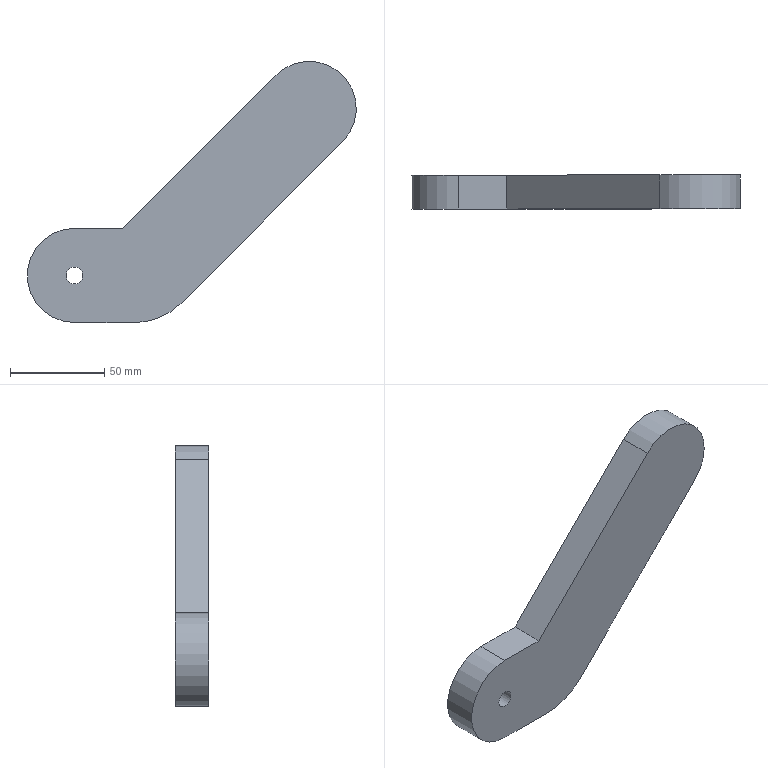Part | STEP file | Leg_right | 1 solid | 10 faces | box 174.595 x 18 x 138.64 mm | volume 178903 mm3 | plane 6 | cylinder 4 | commonest cylinder face diameters 50 x2 9 x1 70 x1
STEP:
#1=CARTESIAN_POINT('',(0.,0.,0.));
#2=DIRECTION('',(0.,0.,1.));
#3=DIRECTION('',(1.,0.,0.));
#4=AXIS2_PLACEMENT_3D('',#1,#2,#3);
#5=CARTESIAN_POINT('',(0.,0.,25.));
#6=VERTEX_POINT('',#5);
#7=CARTESIAN_POINT('',(0.,0.,-25.));
#8=VERTEX_POINT('',#7);
#9=CARTESIAN_POINT('',(0.,0.,0.));
#10=DIRECTION('',(0.,-1.,0.));
#11=DIRECTION('',(1.,0.,0.));
#12=AXIS2_PLACEMENT_3D('',#9,#10,#11);
#13=CIRCLE('',#12,25.);
#14=CARTESIAN_POINT('',(0.,0.,0.));
#15=DIRECTION('',(0.,1.,0.));
#16=DIRECTION('',(1.,0.,0.));
#17=AXIS2_PLACEMENT_3D('',#14,#15,#16);
#18=CYLINDRICAL_SURFACE('',#17,25.);
#19=CARTESIAN_POINT('',(6.283,0.));
#20=DIRECTION('',(-1.,0.));
#21=VECTOR('',#20,1.);
#22=LINE('',#19,#21);
#23=(GEOMETRIC_REPRESENTATION_CONTEXT(2)PARAMETRIC_REPRESENTATION_CONTEXT()REPRESENTATION_CONTEXT('',''));
#24=DEFINITIONAL_REPRESENTATION('',(#22),#23);
#25=PCURVE('',#18,#24);
#26=CARTESIAN_POINT('',(62.213,0.,35.66));
#27=DIRECTION('',(0.,1.,0.));
#28=DIRECTION('',(0.,0.,1.));
#29=AXIS2_PLACEMENT_3D('',#26,#27,#28);
#30=PLANE('',#29);
#31=CARTESIAN_POINT('',(-35.66,-37.213));
#32=CARTESIAN_POINT('',(7.641,-37.213));
#33=CARTESIAN_POINT('',(-14.009,-74.713));
#34=CARTESIAN_POINT('',(-35.66,-112.213));
#35=CARTESIAN_POINT('',(-57.311,-74.713));
#36=CARTESIAN_POINT('',(-78.961,-37.213));
#37=CARTESIAN_POINT('',(-35.66,-37.213));
#38=(BOUNDED_CURVE()B_SPLINE_CURVE(2,(#31,#32,#33,#34,#35,#36,#37),.UNSPECIFIED.,.T.,.F.)B_SPLINE_CURVE_WITH_KNOTS((1,2,2,2,2,1),(-2.094,0.,2.094,4.189,6.283,8.378),.UNSPECIFIED.)CURVE()GEOMETRIC_REPRESENTATION_ITEM()RATIONAL_B_SPLINE_CURVE((1.,0.5,1.,0.5,1.,0.5,1.))REPRESENTATION_ITEM(''));
#39=(GEOMETRIC_REPRESENTATION_CONTEXT(2)PARAMETRIC_REPRESENTATION_CONTEXT()REPRESENTATION_CONTEXT('',''));
#40=DEFINITIONAL_REPRESENTATION('',(#38),#39);
#41=PCURVE('',#30,#40);
#42=SURFACE_CURVE('',#13,(#25,#41),.PCURVE_S1.);
#43=EDGE_CURVE('',#6,#8,#42,.T.);
#44=ORIENTED_EDGE('',*,*,#43,.T.);
#45=CARTESIAN_POINT('',(0.,-18.,-25.));
#46=VERTEX_POINT('',#45);
#47=CARTESIAN_POINT('',(0.,0.,-25.));
#48=DIRECTION('',(0.,-1.,0.));
#49=VECTOR('',#48,1.);
#50=LINE('',#47,#49);
#51=CARTESIAN_POINT('',(1.571,0.));
#52=DIRECTION('',(0.,-1.));
#53=VECTOR('',#52,1.);
#54=LINE('',#51,#53);
#55=(GEOMETRIC_REPRESENTATION_CONTEXT(2)PARAMETRIC_REPRESENTATION_CONTEXT()REPRESENTATION_CONTEXT('',''));
#56=DEFINITIONAL_REPRESENTATION('',(#54),#55);
#57=PCURVE('',#18,#56);
#58=CARTESIAN_POINT('',(31.813,0.,-25.));
#59=DIRECTION('',(0.,0.,-1.));
#60=DIRECTION('',(-1.,0.,0.));
#61=AXIS2_PLACEMENT_3D('',#58,#59,#60);
#62=PLANE('',#61);
#63=CARTESIAN_POINT('',(31.813,0.));
#64=DIRECTION('',(0.,-1.));
#65=VECTOR('',#64,1.);
#66=LINE('',#63,#65);
#67=(GEOMETRIC_REPRESENTATION_CONTEXT(2)PARAMETRIC_REPRESENTATION_CONTEXT()REPRESENTATION_CONTEXT('',''));
#68=DEFINITIONAL_REPRESENTATION('',(#66),#67);
#69=PCURVE('',#62,#68);
#70=SURFACE_CURVE('',#50,(#57,#69),.PCURVE_S1.);
#71=EDGE_CURVE('',#8,#46,#70,.T.);
#72=ORIENTED_EDGE('',*,*,#71,.T.);
#73=CARTESIAN_POINT('',(0.,-18.,25.));
#74=VERTEX_POINT('',#73);
#75=CARTESIAN_POINT('',(0.,-18.,0.));
#76=DIRECTION('',(0.,-1.,0.));
#77=DIRECTION('',(1.,0.,0.));
#78=AXIS2_PLACEMENT_3D('',#75,#76,#77);
#79=CIRCLE('',#78,25.);
#80=CARTESIAN_POINT('',(6.283,-18.));
#81=DIRECTION('',(-1.,0.));
#82=VECTOR('',#81,1.);
#83=LINE('',#80,#82);
#84=(GEOMETRIC_REPRESENTATION_CONTEXT(2)PARAMETRIC_REPRESENTATION_CONTEXT()REPRESENTATION_CONTEXT('',''));
#85=DEFINITIONAL_REPRESENTATION('',(#83),#84);
#86=PCURVE('',#18,#85);
#87=CARTESIAN_POINT('',(62.213,-18.,35.66));
#88=DIRECTION('',(0.,1.,0.));
#89=DIRECTION('',(0.,0.,1.));
#90=AXIS2_PLACEMENT_3D('',#87,#88,#89);
#91=PLANE('',#90);
#92=CARTESIAN_POINT('',(-35.66,-37.213));
#93=CARTESIAN_POINT('',(7.641,-37.213));
#94=CARTESIAN_POINT('',(-14.009,-74.713));
#95=CARTESIAN_POINT('',(-35.66,-112.213));
#96=CARTESIAN_POINT('',(-57.311,-74.713));
#97=CARTESIAN_POINT('',(-78.961,-37.213));
#98=CARTESIAN_POINT('',(-35.66,-37.213));
#99=(BOUNDED_CURVE()B_SPLINE_CURVE(2,(#92,#93,#94,#95,#96,#97,#98),.UNSPECIFIED.,.T.,.F.)B_SPLINE_CURVE_WITH_KNOTS((1,2,2,2,2,1),(-2.094,0.,2.094,4.189,6.283,8.378),.UNSPECIFIED.)CURVE()GEOMETRIC_REPRESENTATION_ITEM()RATIONAL_B_SPLINE_CURVE((1.,0.5,1.,0.5,1.,0.5,1.))REPRESENTATION_ITEM(''));
#100=(GEOMETRIC_REPRESENTATION_CONTEXT(2)PARAMETRIC_REPRESENTATION_CONTEXT()REPRESENTATION_CONTEXT('',''));
#101=DEFINITIONAL_REPRESENTATION('',(#99),#100);
#102=PCURVE('',#91,#101);
#103=SURFACE_CURVE('',#79,(#86,#102),.PCURVE_S1.);
#104=EDGE_CURVE('',#74,#46,#103,.T.);
#105=ORIENTED_EDGE('',*,*,#104,.F.);
#106=CARTESIAN_POINT('',(0.,0.,25.));
#107=DIRECTION('',(0.,-1.,0.));
#108=VECTOR('',#107,1.);
#109=LINE('',#106,#108);
#110=CARTESIAN_POINT('',(4.712,0.));
#111=DIRECTION('',(0.,-1.));
#112=VECTOR('',#111,1.);
#113=LINE('',#110,#112);
#114=(GEOMETRIC_REPRESENTATION_CONTEXT(2)PARAMETRIC_REPRESENTATION_CONTEXT()REPRESENTATION_CONTEXT('',''));
#115=DEFINITIONAL_REPRESENTATION('',(#113),#114);
#116=PCURVE('',#18,#115);
#117=CARTESIAN_POINT('',(0.,0.,25.));
#118=DIRECTION('',(0.,0.,1.));
#119=DIRECTION('',(1.,0.,0.));
#120=AXIS2_PLACEMENT_3D('',#117,#118,#119);
#121=PLANE('',#120);
#122=CARTESIAN_POINT('',(0.,0.));
#123=DIRECTION('',(0.,-1.));
#124=VECTOR('',#123,1.);
#125=LINE('',#122,#124);
#126=(GEOMETRIC_REPRESENTATION_CONTEXT(2)PARAMETRIC_REPRESENTATION_CONTEXT()REPRESENTATION_CONTEXT('',''));
#127=DEFINITIONAL_REPRESENTATION('',(#125),#126);
#128=PCURVE('',#121,#127);
#129=SURFACE_CURVE('',#109,(#116,#128),.PCURVE_S1.);
#130=EDGE_CURVE('',#6,#74,#129,.T.);
#131=ORIENTED_EDGE('',*,*,#130,.F.);
#132=EDGE_LOOP('',(#44,#72,#105,#131));
#133=FACE_BOUND('',#132,.T.);
#134=ADVANCED_FACE('',(#133),#18,.T.);
#135=CARTESIAN_POINT('',(31.813,0.,-25.));
#136=VERTEX_POINT('',#135);
#137=CARTESIAN_POINT('',(31.813,-18.,-25.));
#138=VERTEX_POINT('',#137);
#139=CARTESIAN_POINT('',(31.813,0.,-25.));
#140=DIRECTION('',(0.,-1.,0.));
#141=VECTOR('',#140,1.);
#142=LINE('',#139,#141);
#143=CARTESIAN_POINT('',(0.,0.));
#144=DIRECTION('',(0.,-1.));
#145=VECTOR('',#144,1.);
#146=LINE('',#143,#145);
#147=(GEOMETRIC_REPRESENTATION_CONTEXT(2)PARAMETRIC_REPRESENTATION_CONTEXT()REPRESENTATION_CONTEXT('',''));
#148=DEFINITIONAL_REPRESENTATION('',(#146),#147);
#149=PCURVE('',#62,#148);
#150=CARTESIAN_POINT('',(31.813,0.,10.));
#151=DIRECTION('',(0.,1.,0.));
#152=DIRECTION('',(1.,0.,0.));
#153=AXIS2_PLACEMENT_3D('',#150,#151,#152);
#154=CYLINDRICAL_SURFACE('',#153,35.);
#155=CARTESIAN_POINT('',(1.571,0.));
#156=DIRECTION('',(0.,-1.));
#157=VECTOR('',#156,1.);
#158=LINE('',#155,#157);
#159=(GEOMETRIC_REPRESENTATION_CONTEXT(2)PARAMETRIC_REPRESENTATION_CONTEXT()REPRESENTATION_CONTEXT('',''));
#160=DEFINITIONAL_REPRESENTATION('',(#158),#159);
#161=PCURVE('',#154,#160);
#162=SURFACE_CURVE('',#142,(#149,#161),.PCURVE_S1.);
#163=EDGE_CURVE('',#136,#138,#162,.T.);
#164=ORIENTED_EDGE('',*,*,#163,.T.);
#165=CARTESIAN_POINT('',(31.813,-18.,-25.));
#166=DIRECTION('',(-1.,0.,0.));
#167=VECTOR('',#166,1.);
#168=LINE('',#165,#167);
#169=CARTESIAN_POINT('',(0.,-18.));
#170=DIRECTION('',(1.,0.));
#171=VECTOR('',#170,1.);
#172=LINE('',#169,#171);
#173=(GEOMETRIC_REPRESENTATION_CONTEXT(2)PARAMETRIC_REPRESENTATION_CONTEXT()REPRESENTATION_CONTEXT('',''));
#174=DEFINITIONAL_REPRESENTATION('',(#172),#173);
#175=PCURVE('',#62,#174);
#176=CARTESIAN_POINT('',(-60.66,-30.4));
#177=DIRECTION('',(0.,-1.));
#178=VECTOR('',#177,1.);
#179=LINE('',#176,#178);
#180=(GEOMETRIC_REPRESENTATION_CONTEXT(2)PARAMETRIC_REPRESENTATION_CONTEXT()REPRESENTATION_CONTEXT('',''));
#181=DEFINITIONAL_REPRESENTATION('',(#179),#180);
#182=PCURVE('',#91,#181);
#183=SURFACE_CURVE('',#168,(#175,#182),.PCURVE_S1.);
#184=EDGE_CURVE('',#138,#46,#183,.T.);
#185=ORIENTED_EDGE('',*,*,#184,.T.);
#186=ORIENTED_EDGE('',*,*,#71,.F.);
#187=CARTESIAN_POINT('',(31.813,0.,-25.));
#188=DIRECTION('',(-1.,0.,0.));
#189=VECTOR('',#188,1.);
#190=LINE('',#187,#189);
#191=CARTESIAN_POINT('',(0.,0.));
#192=DIRECTION('',(1.,0.));
#193=VECTOR('',#192,1.);
#194=LINE('',#191,#193);
#195=(GEOMETRIC_REPRESENTATION_CONTEXT(2)PARAMETRIC_REPRESENTATION_CONTEXT()REPRESENTATION_CONTEXT('',''));
#196=DEFINITIONAL_REPRESENTATION('',(#194),#195);
#197=PCURVE('',#62,#196);
#198=CARTESIAN_POINT('',(-60.66,-30.4));
#199=DIRECTION('',(0.,-1.));
#200=VECTOR('',#199,1.);
#201=LINE('',#198,#200);
#202=(GEOMETRIC_REPRESENTATION_CONTEXT(2)PARAMETRIC_REPRESENTATION_CONTEXT()REPRESENTATION_CONTEXT('',''));
#203=DEFINITIONAL_REPRESENTATION('',(#201),#202);
#204=PCURVE('',#30,#203);
#205=SURFACE_CURVE('',#190,(#197,#204),.PCURVE_S1.);
#206=EDGE_CURVE('',#136,#8,#205,.T.);
#207=ORIENTED_EDGE('',*,*,#206,.F.);
#208=EDGE_LOOP('',(#164,#185,#186,#207));
#209=FACE_BOUND('',#208,.T.);
#210=ADVANCED_FACE('',(#209),#62,.T.);
#211=CARTESIAN_POINT('',(56.562,0.,-14.749));
#212=VERTEX_POINT('',#211);
#213=CARTESIAN_POINT('',(31.813,0.,10.));
#214=DIRECTION('',(0.,-1.,0.));
#215=DIRECTION('',(1.,0.,0.));
#216=AXIS2_PLACEMENT_3D('',#213,#214,#215);
#217=CIRCLE('',#216,35.);
#218=CARTESIAN_POINT('',(6.283,0.));
#219=DIRECTION('',(-1.,0.));
#220=VECTOR('',#219,1.);
#221=LINE('',#218,#220);
#222=(GEOMETRIC_REPRESENTATION_CONTEXT(2)PARAMETRIC_REPRESENTATION_CONTEXT()REPRESENTATION_CONTEXT('',''));
#223=DEFINITIONAL_REPRESENTATION('',(#221),#222);
#224=PCURVE('',#154,#223);
#225=CARTESIAN_POINT('',(-25.66,4.6));
#226=CARTESIAN_POINT('',(34.962,4.6));
#227=CARTESIAN_POINT('',(4.651,-47.9));
#228=CARTESIAN_POINT('',(-25.66,-100.4));
#229=CARTESIAN_POINT('',(-55.971,-47.9));
#230=CARTESIAN_POINT('',(-86.282,4.6));
#231=CARTESIAN_POINT('',(-25.66,4.6));
#232=(BOUNDED_CURVE()B_SPLINE_CURVE(2,(#225,#226,#227,#228,#229,#230,#231),.UNSPECIFIED.,.T.,.F.)B_SPLINE_CURVE_WITH_KNOTS((1,2,2,2,2,1),(-2.094,0.,2.094,4.189,6.283,8.378),.UNSPECIFIED.)CURVE()GEOMETRIC_REPRESENTATION_ITEM()RATIONAL_B_SPLINE_CURVE((1.,0.5,1.,0.5,1.,0.5,1.))REPRESENTATION_ITEM(''));
#233=(GEOMETRIC_REPRESENTATION_CONTEXT(2)PARAMETRIC_REPRESENTATION_CONTEXT()REPRESENTATION_CONTEXT('',''));
#234=DEFINITIONAL_REPRESENTATION('',(#232),#233);
#235=PCURVE('',#30,#234);
#236=SURFACE_CURVE('',#217,(#224,#235),.PCURVE_S1.);
#237=EDGE_CURVE('',#136,#212,#236,.T.);
#238=ORIENTED_EDGE('',*,*,#237,.T.);
#239=CARTESIAN_POINT('',(56.562,-18.,-14.749));
#240=VERTEX_POINT('',#239);
#241=CARTESIAN_POINT('',(56.562,0.,-14.749));
#242=DIRECTION('',(0.,-1.,0.));
#243=VECTOR('',#242,1.);
#244=LINE('',#241,#243);
#245=CARTESIAN_POINT('',(0.7854,0.));
#246=DIRECTION('',(0.,-1.));
#247=VECTOR('',#246,1.);
#248=LINE('',#245,#247);
#249=(GEOMETRIC_REPRESENTATION_CONTEXT(2)PARAMETRIC_REPRESENTATION_CONTEXT()REPRESENTATION_CONTEXT('',''));
#250=DEFINITIONAL_REPRESENTATION('',(#248),#249);
#251=PCURVE('',#154,#250);
#252=CARTESIAN_POINT('',(142.273,0.,70.962));
#253=DIRECTION('',(0.7071,0.,-0.7071));
#254=DIRECTION('',(-0.7071,0.,-0.7071));
#255=AXIS2_PLACEMENT_3D('',#252,#253,#254);
#256=PLANE('',#255);
#257=CARTESIAN_POINT('',(121.213,0.));
#258=DIRECTION('',(0.,-1.));
#259=VECTOR('',#258,1.);
#260=LINE('',#257,#259);
#261=(GEOMETRIC_REPRESENTATION_CONTEXT(2)PARAMETRIC_REPRESENTATION_CONTEXT()REPRESENTATION_CONTEXT('',''));
#262=DEFINITIONAL_REPRESENTATION('',(#260),#261);
#263=PCURVE('',#256,#262);
#264=SURFACE_CURVE('',#244,(#251,#263),.PCURVE_S1.);
#265=EDGE_CURVE('',#212,#240,#264,.T.);
#266=ORIENTED_EDGE('',*,*,#265,.T.);
#267=CARTESIAN_POINT('',(31.813,-18.,10.));
#268=DIRECTION('',(0.,-1.,0.));
#269=DIRECTION('',(1.,0.,0.));
#270=AXIS2_PLACEMENT_3D('',#267,#268,#269);
#271=CIRCLE('',#270,35.);
#272=CARTESIAN_POINT('',(6.283,-18.));
#273=DIRECTION('',(-1.,0.));
#274=VECTOR('',#273,1.);
#275=LINE('',#272,#274);
#276=(GEOMETRIC_REPRESENTATION_CONTEXT(2)PARAMETRIC_REPRESENTATION_CONTEXT()REPRESENTATION_CONTEXT('',''));
#277=DEFINITIONAL_REPRESENTATION('',(#275),#276);
#278=PCURVE('',#154,#277);
#279=CARTESIAN_POINT('',(-25.66,4.6));
#280=CARTESIAN_POINT('',(34.962,4.6));
#281=CARTESIAN_POINT('',(4.651,-47.9));
#282=CARTESIAN_POINT('',(-25.66,-100.4));
#283=CARTESIAN_POINT('',(-55.971,-47.9));
#284=CARTESIAN_POINT('',(-86.282,4.6));
#285=CARTESIAN_POINT('',(-25.66,4.6));
#286=(BOUNDED_CURVE()B_SPLINE_CURVE(2,(#279,#280,#281,#282,#283,#284,#285),.UNSPECIFIED.,.T.,.F.)B_SPLINE_CURVE_WITH_KNOTS((1,2,2,2,2,1),(-2.094,0.,2.094,4.189,6.283,8.378),.UNSPECIFIED.)CURVE()GEOMETRIC_REPRESENTATION_ITEM()RATIONAL_B_SPLINE_CURVE((1.,0.5,1.,0.5,1.,0.5,1.))REPRESENTATION_ITEM(''));
#287=(GEOMETRIC_REPRESENTATION_CONTEXT(2)PARAMETRIC_REPRESENTATION_CONTEXT()REPRESENTATION_CONTEXT('',''));
#288=DEFINITIONAL_REPRESENTATION('',(#286),#287);
#289=PCURVE('',#91,#288);
#290=SURFACE_CURVE('',#271,(#278,#289),.PCURVE_S1.);
#291=EDGE_CURVE('',#138,#240,#290,.T.);
#292=ORIENTED_EDGE('',*,*,#291,.F.);
#293=ORIENTED_EDGE('',*,*,#163,.F.);
#294=EDGE_LOOP('',(#238,#266,#292,#293));
#295=FACE_BOUND('',#294,.T.);
#296=ADVANCED_FACE('',(#295),#154,.T.);
#297=CARTESIAN_POINT('',(142.273,0.,70.962));
#298=VERTEX_POINT('',#297);
#299=CARTESIAN_POINT('',(142.273,-18.,70.962));
#300=VERTEX_POINT('',#299);
#301=CARTESIAN_POINT('',(142.273,0.,70.962));
#302=DIRECTION('',(0.,-1.,0.));
#303=VECTOR('',#302,1.);
#304=LINE('',#301,#303);
#305=CARTESIAN_POINT('',(0.,0.));
#306=DIRECTION('',(0.,-1.));
#307=VECTOR('',#306,1.);
#308=LINE('',#305,#307);
#309=(GEOMETRIC_REPRESENTATION_CONTEXT(2)PARAMETRIC_REPRESENTATION_CONTEXT()REPRESENTATION_CONTEXT('',''));
#310=DEFINITIONAL_REPRESENTATION('',(#308),#309);
#311=PCURVE('',#256,#310);
#312=CARTESIAN_POINT('',(124.595,0.,88.64));
#313=DIRECTION('',(0.,1.,0.));
#314=DIRECTION('',(1.,0.,0.));
#315=AXIS2_PLACEMENT_3D('',#312,#313,#314);
#316=CYLINDRICAL_SURFACE('',#315,25.);
#317=CARTESIAN_POINT('',(7.069,0.));
#318=DIRECTION('',(0.,-1.));
#319=VECTOR('',#318,1.);
#320=LINE('',#317,#319);
#321=(GEOMETRIC_REPRESENTATION_CONTEXT(2)PARAMETRIC_REPRESENTATION_CONTEXT()REPRESENTATION_CONTEXT('',''));
#322=DEFINITIONAL_REPRESENTATION('',(#320),#321);
#323=PCURVE('',#316,#322);
#324=SURFACE_CURVE('',#304,(#311,#323),.PCURVE_S1.);
#325=EDGE_CURVE('',#298,#300,#324,.T.);
#326=ORIENTED_EDGE('',*,*,#325,.T.);
#327=CARTESIAN_POINT('',(142.273,-18.,70.962));
#328=DIRECTION('',(-0.7071,0.,-0.7071));
#329=VECTOR('',#328,1.);
#330=LINE('',#327,#329);
#331=CARTESIAN_POINT('',(0.,-18.));
#332=DIRECTION('',(1.,0.));
#333=VECTOR('',#332,1.);
#334=LINE('',#331,#333);
#335=(GEOMETRIC_REPRESENTATION_CONTEXT(2)PARAMETRIC_REPRESENTATION_CONTEXT()REPRESENTATION_CONTEXT('',''));
#336=DEFINITIONAL_REPRESENTATION('',(#334),#335);
#337=PCURVE('',#256,#336);
#338=CARTESIAN_POINT('',(35.302,80.059));
#339=DIRECTION('',(-0.7071,-0.7071));
#340=VECTOR('',#339,1.);
#341=LINE('',#338,#340);
#342=(GEOMETRIC_REPRESENTATION_CONTEXT(2)PARAMETRIC_REPRESENTATION_CONTEXT()REPRESENTATION_CONTEXT('',''));
#343=DEFINITIONAL_REPRESENTATION('',(#341),#342);
#344=PCURVE('',#91,#343);
#345=SURFACE_CURVE('',#330,(#337,#344),.PCURVE_S1.);
#346=EDGE_CURVE('',#300,#240,#345,.T.);
#347=ORIENTED_EDGE('',*,*,#346,.T.);
#348=ORIENTED_EDGE('',*,*,#265,.F.);
#349=CARTESIAN_POINT('',(142.273,0.,70.962));
#350=DIRECTION('',(-0.7071,0.,-0.7071));
#351=VECTOR('',#350,1.);
#352=LINE('',#349,#351);
#353=CARTESIAN_POINT('',(0.,0.));
#354=DIRECTION('',(1.,0.));
#355=VECTOR('',#354,1.);
#356=LINE('',#353,#355);
#357=(GEOMETRIC_REPRESENTATION_CONTEXT(2)PARAMETRIC_REPRESENTATION_CONTEXT()REPRESENTATION_CONTEXT('',''));
#358=DEFINITIONAL_REPRESENTATION('',(#356),#357);
#359=PCURVE('',#256,#358);
#360=CARTESIAN_POINT('',(35.302,80.059));
#361=DIRECTION('',(-0.7071,-0.7071));
#362=VECTOR('',#361,1.);
#363=LINE('',#360,#362);
#364=(GEOMETRIC_REPRESENTATION_CONTEXT(2)PARAMETRIC_REPRESENTATION_CONTEXT()REPRESENTATION_CONTEXT('',''));
#365=DEFINITIONAL_REPRESENTATION('',(#363),#364);
#366=PCURVE('',#30,#365);
#367=SURFACE_CURVE('',#352,(#359,#366),.PCURVE_S1.);
#368=EDGE_CURVE('',#298,#212,#367,.T.);
#369=ORIENTED_EDGE('',*,*,#368,.F.);
#370=EDGE_LOOP('',(#326,#347,#348,#369));
#371=FACE_BOUND('',#370,.T.);
#372=ADVANCED_FACE('',(#371),#256,.T.);
#373=CARTESIAN_POINT('',(106.917,0.,106.317));
#374=VERTEX_POINT('',#373);
#375=CARTESIAN_POINT('',(124.595,0.,88.64));
#376=DIRECTION('',(0.,-1.,0.));
#377=DIRECTION('',(1.,0.,0.));
#378=AXIS2_PLACEMENT_3D('',#375,#376,#377);
#379=CIRCLE('',#378,25.);
#380=CARTESIAN_POINT('',(12.566,0.));
#381=DIRECTION('',(-1.,0.));
#382=VECTOR('',#381,1.);
#383=LINE('',#380,#382);
#384=(GEOMETRIC_REPRESENTATION_CONTEXT(2)PARAMETRIC_REPRESENTATION_CONTEXT()REPRESENTATION_CONTEXT('',''));
#385=DEFINITIONAL_REPRESENTATION('',(#383),#384);
#386=PCURVE('',#316,#385);
#387=CARTESIAN_POINT('',(52.98,87.382));
#388=CARTESIAN_POINT('',(96.281,87.382));
#389=CARTESIAN_POINT('',(74.63,49.882));
#390=CARTESIAN_POINT('',(52.98,12.382));
#391=CARTESIAN_POINT('',(31.329,49.882));
#392=CARTESIAN_POINT('',(9.678,87.382));
#393=CARTESIAN_POINT('',(52.98,87.382));
#394=(BOUNDED_CURVE()B_SPLINE_CURVE(2,(#387,#388,#389,#390,#391,#392,#393),.UNSPECIFIED.,.T.,.F.)B_SPLINE_CURVE_WITH_KNOTS((1,2,2,2,2,1),(-2.094,0.,2.094,4.189,6.283,8.378),.UNSPECIFIED.)CURVE()GEOMETRIC_REPRESENTATION_ITEM()RATIONAL_B_SPLINE_CURVE((1.,0.5,1.,0.5,1.,0.5,1.))REPRESENTATION_ITEM(''));
#395=(GEOMETRIC_REPRESENTATION_CONTEXT(2)PARAMETRIC_REPRESENTATION_CONTEXT()REPRESENTATION_CONTEXT('',''));
#396=DEFINITIONAL_REPRESENTATION('',(#394),#395);
#397=PCURVE('',#30,#396);
#398=SURFACE_CURVE('',#379,(#386,#397),.PCURVE_S1.);
#399=EDGE_CURVE('',#298,#374,#398,.T.);
#400=ORIENTED_EDGE('',*,*,#399,.T.);
#401=CARTESIAN_POINT('',(106.917,-18.,106.317));
#402=VERTEX_POINT('',#401);
#403=CARTESIAN_POINT('',(106.917,0.,106.317));
#404=DIRECTION('',(0.,-1.,0.));
#405=VECTOR('',#404,1.);
#406=LINE('',#403,#405);
#407=CARTESIAN_POINT('',(3.927,0.));
#408=DIRECTION('',(0.,-1.));
#409=VECTOR('',#408,1.);
#410=LINE('',#407,#409);
#411=(GEOMETRIC_REPRESENTATION_CONTEXT(2)PARAMETRIC_REPRESENTATION_CONTEXT()REPRESENTATION_CONTEXT('',''));
#412=DEFINITIONAL_REPRESENTATION('',(#410),#411);
#413=PCURVE('',#316,#412);
#414=CARTESIAN_POINT('',(25.6,0.,25.));
#415=DIRECTION('',(-0.7071,0.,0.7071));
#416=DIRECTION('',(0.7071,0.,0.7071));
#417=AXIS2_PLACEMENT_3D('',#414,#415,#416);
#418=PLANE('',#417);
#419=CARTESIAN_POINT('',(115.,0.));
#420=DIRECTION('',(0.,-1.));
#421=VECTOR('',#420,1.);
#422=LINE('',#419,#421);
#423=(GEOMETRIC_REPRESENTATION_CONTEXT(2)PARAMETRIC_REPRESENTATION_CONTEXT()REPRESENTATION_CONTEXT('',''));
#424=DEFINITIONAL_REPRESENTATION('',(#422),#423);
#425=PCURVE('',#418,#424);
#426=SURFACE_CURVE('',#406,(#413,#425),.PCURVE_S1.);
#427=EDGE_CURVE('',#374,#402,#426,.T.);
#428=ORIENTED_EDGE('',*,*,#427,.T.);
#429=CARTESIAN_POINT('',(124.595,-18.,88.64));
#430=DIRECTION('',(0.,-1.,0.));
#431=DIRECTION('',(1.,0.,0.));
#432=AXIS2_PLACEMENT_3D('',#429,#430,#431);
#433=CIRCLE('',#432,25.);
#434=CARTESIAN_POINT('',(12.566,-18.));
#435=DIRECTION('',(-1.,0.));
#436=VECTOR('',#435,1.);
#437=LINE('',#434,#436);
#438=(GEOMETRIC_REPRESENTATION_CONTEXT(2)PARAMETRIC_REPRESENTATION_CONTEXT()REPRESENTATION_CONTEXT('',''));
#439=DEFINITIONAL_REPRESENTATION('',(#437),#438);
#440=PCURVE('',#316,#439);
#441=CARTESIAN_POINT('',(52.98,87.382));
#442=CARTESIAN_POINT('',(96.281,87.382));
#443=CARTESIAN_POINT('',(74.63,49.882));
#444=CARTESIAN_POINT('',(52.98,12.382));
#445=CARTESIAN_POINT('',(31.329,49.882));
#446=CARTESIAN_POINT('',(9.678,87.382));
#447=CARTESIAN_POINT('',(52.98,87.382));
#448=(BOUNDED_CURVE()B_SPLINE_CURVE(2,(#441,#442,#443,#444,#445,#446,#447),.UNSPECIFIED.,.T.,.F.)B_SPLINE_CURVE_WITH_KNOTS((1,2,2,2,2,1),(-2.094,0.,2.094,4.189,6.283,8.378),.UNSPECIFIED.)CURVE()GEOMETRIC_REPRESENTATION_ITEM()RATIONAL_B_SPLINE_CURVE((1.,0.5,1.,0.5,1.,0.5,1.))REPRESENTATION_ITEM(''));
#449=(GEOMETRIC_REPRESENTATION_CONTEXT(2)PARAMETRIC_REPRESENTATION_CONTEXT()REPRESENTATION_CONTEXT('',''));
#450=DEFINITIONAL_REPRESENTATION('',(#448),#449);
#451=PCURVE('',#91,#450);
#452=SURFACE_CURVE('',#433,(#440,#451),.PCURVE_S1.);
#453=EDGE_CURVE('',#300,#402,#452,.T.);
#454=ORIENTED_EDGE('',*,*,#453,.F.);
#455=ORIENTED_EDGE('',*,*,#325,.F.);
#456=EDGE_LOOP('',(#400,#428,#454,#455));
#457=FACE_BOUND('',#456,.T.);
#458=ADVANCED_FACE('',(#457),#316,.T.);
#459=CARTESIAN_POINT('',(25.6,0.,25.));
#460=VERTEX_POINT('',#459);
#461=CARTESIAN_POINT('',(25.6,-18.,25.));
#462=VERTEX_POINT('',#461);
#463=CARTESIAN_POINT('',(25.6,0.,25.));
#464=DIRECTION('',(0.,-1.,0.));
#465=VECTOR('',#464,1.);
#466=LINE('',#463,#465);
#467=CARTESIAN_POINT('',(0.,0.));
#468=DIRECTION('',(0.,-1.));
#469=VECTOR('',#468,1.);
#470=LINE('',#467,#469);
#471=(GEOMETRIC_REPRESENTATION_CONTEXT(2)PARAMETRIC_REPRESENTATION_CONTEXT()REPRESENTATION_CONTEXT('',''));
#472=DEFINITIONAL_REPRESENTATION('',(#470),#471);
#473=PCURVE('',#418,#472);
#474=CARTESIAN_POINT('',(25.6,0.));
#475=DIRECTION('',(0.,-1.));
#476=VECTOR('',#475,1.);
#477=LINE('',#474,#476);
#478=(GEOMETRIC_REPRESENTATION_CONTEXT(2)PARAMETRIC_REPRESENTATION_CONTEXT()REPRESENTATION_CONTEXT('',''));
#479=DEFINITIONAL_REPRESENTATION('',(#477),#478);
#480=PCURVE('',#121,#479);
#481=SURFACE_CURVE('',#466,(#473,#480),.PCURVE_S1.);
#482=EDGE_CURVE('',#460,#462,#481,.T.);
#483=ORIENTED_EDGE('',*,*,#482,.T.);
#484=CARTESIAN_POINT('',(25.6,-18.,25.));
#485=DIRECTION('',(0.7071,0.,0.7071));
#486=VECTOR('',#485,1.);
#487=LINE('',#484,#486);
#488=CARTESIAN_POINT('',(0.,-18.));
#489=DIRECTION('',(1.,0.));
#490=VECTOR('',#489,1.);
#491=LINE('',#488,#490);
#492=(GEOMETRIC_REPRESENTATION_CONTEXT(2)PARAMETRIC_REPRESENTATION_CONTEXT()REPRESENTATION_CONTEXT('',''));
#493=DEFINITIONAL_REPRESENTATION('',(#491),#492);
#494=PCURVE('',#418,#493);
#495=CARTESIAN_POINT('',(-10.66,-36.613));
#496=DIRECTION('',(0.7071,0.7071));
#497=VECTOR('',#496,1.);
#498=LINE('',#495,#497);
#499=(GEOMETRIC_REPRESENTATION_CONTEXT(2)PARAMETRIC_REPRESENTATION_CONTEXT()REPRESENTATION_CONTEXT('',''));
#500=DEFINITIONAL_REPRESENTATION('',(#498),#499);
#501=PCURVE('',#91,#500);
#502=SURFACE_CURVE('',#487,(#494,#501),.PCURVE_S1.);
#503=EDGE_CURVE('',#462,#402,#502,.T.);
#504=ORIENTED_EDGE('',*,*,#503,.T.);
#505=ORIENTED_EDGE('',*,*,#427,.F.);
#506=CARTESIAN_POINT('',(25.6,0.,25.));
#507=DIRECTION('',(0.7071,0.,0.7071));
#508=VECTOR('',#507,1.);
#509=LINE('',#506,#508);
#510=CARTESIAN_POINT('',(0.,0.));
#511=DIRECTION('',(1.,0.));
#512=VECTOR('',#511,1.);
#513=LINE('',#510,#512);
#514=(GEOMETRIC_REPRESENTATION_CONTEXT(2)PARAMETRIC_REPRESENTATION_CONTEXT()REPRESENTATION_CONTEXT('',''));
#515=DEFINITIONAL_REPRESENTATION('',(#513),#514);
#516=PCURVE('',#418,#515);
#517=CARTESIAN_POINT('',(-10.66,-36.613));
#518=DIRECTION('',(0.7071,0.7071));
#519=VECTOR('',#518,1.);
#520=LINE('',#517,#519);
#521=(GEOMETRIC_REPRESENTATION_CONTEXT(2)PARAMETRIC_REPRESENTATION_CONTEXT()REPRESENTATION_CONTEXT('',''));
#522=DEFINITIONAL_REPRESENTATION('',(#520),#521);
#523=PCURVE('',#30,#522);
#524=SURFACE_CURVE('',#509,(#516,#523),.PCURVE_S1.);
#525=EDGE_CURVE('',#460,#374,#524,.T.);
#526=ORIENTED_EDGE('',*,*,#525,.F.);
#527=EDGE_LOOP('',(#483,#504,#505,#526));
#528=FACE_BOUND('',#527,.T.);
#529=ADVANCED_FACE('',(#528),#418,.T.);
#530=ORIENTED_EDGE('',*,*,#130,.T.);
#531=CARTESIAN_POINT('',(0.,-18.,25.));
#532=DIRECTION('',(1.,0.,0.));
#533=VECTOR('',#532,1.);
#534=LINE('',#531,#533);
#535=CARTESIAN_POINT('',(0.,-18.));
#536=DIRECTION('',(1.,0.));
#537=VECTOR('',#536,1.);
#538=LINE('',#535,#537);
#539=(GEOMETRIC_REPRESENTATION_CONTEXT(2)PARAMETRIC_REPRESENTATION_CONTEXT()REPRESENTATION_CONTEXT('',''));
#540=DEFINITIONAL_REPRESENTATION('',(#538),#539);
#541=PCURVE('',#121,#540);
#542=CARTESIAN_POINT('',(-10.66,-62.213));
#543=DIRECTION('',(0.,1.));
#544=VECTOR('',#543,1.);
#545=LINE('',#542,#544);
#546=(GEOMETRIC_REPRESENTATION_CONTEXT(2)PARAMETRIC_REPRESENTATION_CONTEXT()REPRESENTATION_CONTEXT('',''));
#547=DEFINITIONAL_REPRESENTATION('',(#545),#546);
#548=PCURVE('',#91,#547);
#549=SURFACE_CURVE('',#534,(#541,#548),.PCURVE_S1.);
#550=EDGE_CURVE('',#74,#462,#549,.T.);
#551=ORIENTED_EDGE('',*,*,#550,.T.);
#552=ORIENTED_EDGE('',*,*,#482,.F.);
#553=CARTESIAN_POINT('',(0.,0.,25.));
#554=DIRECTION('',(1.,0.,0.));
#555=VECTOR('',#554,1.);
#556=LINE('',#553,#555);
#557=CARTESIAN_POINT('',(0.,0.));
#558=DIRECTION('',(1.,0.));
#559=VECTOR('',#558,1.);
#560=LINE('',#557,#559);
#561=(GEOMETRIC_REPRESENTATION_CONTEXT(2)PARAMETRIC_REPRESENTATION_CONTEXT()REPRESENTATION_CONTEXT('',''));
#562=DEFINITIONAL_REPRESENTATION('',(#560),#561);
#563=PCURVE('',#121,#562);
#564=CARTESIAN_POINT('',(-10.66,-62.213));
#565=DIRECTION('',(0.,1.));
#566=VECTOR('',#565,1.);
#567=LINE('',#564,#566);
#568=(GEOMETRIC_REPRESENTATION_CONTEXT(2)PARAMETRIC_REPRESENTATION_CONTEXT()REPRESENTATION_CONTEXT('',''));
#569=DEFINITIONAL_REPRESENTATION('',(#567),#568);
#570=PCURVE('',#30,#569);
#571=SURFACE_CURVE('',#556,(#563,#570),.PCURVE_S1.);
#572=EDGE_CURVE('',#6,#460,#571,.T.);
#573=ORIENTED_EDGE('',*,*,#572,.F.);
#574=EDGE_LOOP('',(#530,#551,#552,#573));
#575=FACE_BOUND('',#574,.T.);
#576=ADVANCED_FACE('',(#575),#121,.T.);
#577=CARTESIAN_POINT('',(4.5,0.,0.));
#578=VERTEX_POINT('',#577);
#579=CARTESIAN_POINT('',(0.,0.,0.));
#580=DIRECTION('',(0.,-1.,0.));
#581=DIRECTION('',(1.,0.,0.));
#582=AXIS2_PLACEMENT_3D('',#579,#580,#581);
#583=CIRCLE('',#582,4.5);
#584=CARTESIAN_POINT('',(0.,0.,0.));
#585=DIRECTION('',(0.,1.,0.));
#586=DIRECTION('',(1.,0.,0.));
#587=AXIS2_PLACEMENT_3D('',#584,#585,#586);
#588=CYLINDRICAL_SURFACE('',#587,4.5);
#589=CARTESIAN_POINT('',(6.283,0.));
#590=DIRECTION('',(-1.,0.));
#591=VECTOR('',#590,1.);
#592=LINE('',#589,#591);
#593=(GEOMETRIC_REPRESENTATION_CONTEXT(2)PARAMETRIC_REPRESENTATION_CONTEXT()REPRESENTATION_CONTEXT('',''));
#594=DEFINITIONAL_REPRESENTATION('',(#592),#593);
#595=PCURVE('',#588,#594);
#596=CARTESIAN_POINT('',(-35.66,-57.713));
#597=CARTESIAN_POINT('',(-27.866,-57.713));
#598=CARTESIAN_POINT('',(-31.763,-64.463));
#599=CARTESIAN_POINT('',(-35.66,-71.213));
#600=CARTESIAN_POINT('',(-39.557,-64.463));
#601=CARTESIAN_POINT('',(-43.454,-57.713));
#602=CARTESIAN_POINT('',(-35.66,-57.713));
#603=(BOUNDED_CURVE()B_SPLINE_CURVE(2,(#596,#597,#598,#599,#600,#601,#602),.UNSPECIFIED.,.T.,.F.)B_SPLINE_CURVE_WITH_KNOTS((1,2,2,2,2,1),(-2.094,0.,2.094,4.189,6.283,8.378),.UNSPECIFIED.)CURVE()GEOMETRIC_REPRESENTATION_ITEM()RATIONAL_B_SPLINE_CURVE((1.,0.5,1.,0.5,1.,0.5,1.))REPRESENTATION_ITEM(''));
#604=(GEOMETRIC_REPRESENTATION_CONTEXT(2)PARAMETRIC_REPRESENTATION_CONTEXT()REPRESENTATION_CONTEXT('',''));
#605=DEFINITIONAL_REPRESENTATION('',(#603),#604);
#606=PCURVE('',#30,#605);
#607=SURFACE_CURVE('',#583,(#595,#606),.PCURVE_S1.);
#608=EDGE_CURVE('',#578,#578,#607,.T.);
#609=ORIENTED_EDGE('',*,*,#608,.T.);
#610=CARTESIAN_POINT('',(4.5,-18.,0.));
#611=VERTEX_POINT('',#610);
#612=CARTESIAN_POINT('',(4.5,0.,0.));
#613=DIRECTION('',(0.,-1.,0.));
#614=VECTOR('',#613,1.);
#615=LINE('',#612,#614);
#616=CARTESIAN_POINT('',(0.,0.));
#617=DIRECTION('',(0.,-1.));
#618=VECTOR('',#617,1.);
#619=LINE('',#616,#618);
#620=(GEOMETRIC_REPRESENTATION_CONTEXT(2)PARAMETRIC_REPRESENTATION_CONTEXT()REPRESENTATION_CONTEXT('',''));
#621=DEFINITIONAL_REPRESENTATION('',(#619),#620);
#622=PCURVE('',#588,#621);
#623=CARTESIAN_POINT('',(6.283,0.));
#624=DIRECTION('',(0.,-1.));
#625=VECTOR('',#624,1.);
#626=LINE('',#623,#625);
#627=(GEOMETRIC_REPRESENTATION_CONTEXT(2)PARAMETRIC_REPRESENTATION_CONTEXT()REPRESENTATION_CONTEXT('',''));
#628=DEFINITIONAL_REPRESENTATION('',(#626),#627);
#629=PCURVE('',#588,#628);
#630=SEAM_CURVE('',#615,(#622,#629),.PCURVE_S1.);
#631=EDGE_CURVE('',#578,#611,#630,.T.);
#632=ORIENTED_EDGE('',*,*,#631,.T.);
#633=CARTESIAN_POINT('',(0.,-18.,0.));
#634=DIRECTION('',(0.,-1.,0.));
#635=DIRECTION('',(1.,0.,0.));
#636=AXIS2_PLACEMENT_3D('',#633,#634,#635);
#637=CIRCLE('',#636,4.5);
#638=CARTESIAN_POINT('',(6.283,-18.));
#639=DIRECTION('',(-1.,0.));
#640=VECTOR('',#639,1.);
#641=LINE('',#638,#640);
#642=(GEOMETRIC_REPRESENTATION_CONTEXT(2)PARAMETRIC_REPRESENTATION_CONTEXT()REPRESENTATION_CONTEXT('',''));
#643=DEFINITIONAL_REPRESENTATION('',(#641),#642);
#644=PCURVE('',#588,#643);
#645=CARTESIAN_POINT('',(-35.66,-57.713));
#646=CARTESIAN_POINT('',(-27.866,-57.713));
#647=CARTESIAN_POINT('',(-31.763,-64.463));
#648=CARTESIAN_POINT('',(-35.66,-71.213));
#649=CARTESIAN_POINT('',(-39.557,-64.463));
#650=CARTESIAN_POINT('',(-43.454,-57.713));
#651=CARTESIAN_POINT('',(-35.66,-57.713));
#652=(BOUNDED_CURVE()B_SPLINE_CURVE(2,(#645,#646,#647,#648,#649,#650,#651),.UNSPECIFIED.,.T.,.F.)B_SPLINE_CURVE_WITH_KNOTS((1,2,2,2,2,1),(-2.094,0.,2.094,4.189,6.283,8.378),.UNSPECIFIED.)CURVE()GEOMETRIC_REPRESENTATION_ITEM()RATIONAL_B_SPLINE_CURVE((1.,0.5,1.,0.5,1.,0.5,1.))REPRESENTATION_ITEM(''));
#653=(GEOMETRIC_REPRESENTATION_CONTEXT(2)PARAMETRIC_REPRESENTATION_CONTEXT()REPRESENTATION_CONTEXT('',''));
#654=DEFINITIONAL_REPRESENTATION('',(#652),#653);
#655=PCURVE('',#91,#654);
#656=SURFACE_CURVE('',#637,(#644,#655),.PCURVE_S1.);
#657=EDGE_CURVE('',#611,#611,#656,.T.);
#658=ORIENTED_EDGE('',*,*,#657,.F.);
#659=ORIENTED_EDGE('',*,*,#631,.F.);
#660=EDGE_LOOP('',(#609,#632,#658,#659));
#661=FACE_BOUND('',#660,.F.);
#662=ADVANCED_FACE('',(#661),#588,.F.);
#663=ORIENTED_EDGE('',*,*,#43,.T.);
#664=ORIENTED_EDGE('',*,*,#206,.F.);
#665=ORIENTED_EDGE('',*,*,#237,.T.);
#666=ORIENTED_EDGE('',*,*,#368,.F.);
#667=ORIENTED_EDGE('',*,*,#399,.T.);
#668=ORIENTED_EDGE('',*,*,#525,.F.);
#669=ORIENTED_EDGE('',*,*,#572,.F.);
#670=EDGE_LOOP('',(#663,#664,#665,#666,#667,#668,#669));
#671=FACE_BOUND('',#670,.F.);
#672=ORIENTED_EDGE('',*,*,#608,.T.);
#673=EDGE_LOOP('',(#672));
#674=FACE_BOUND('',#673,.T.);
#675=ADVANCED_FACE('',(#671,#674),#30,.T.);
#676=ORIENTED_EDGE('',*,*,#104,.T.);
#677=ORIENTED_EDGE('',*,*,#184,.F.);
#678=ORIENTED_EDGE('',*,*,#291,.T.);
#679=ORIENTED_EDGE('',*,*,#346,.F.);
#680=ORIENTED_EDGE('',*,*,#453,.T.);
#681=ORIENTED_EDGE('',*,*,#503,.F.);
#682=ORIENTED_EDGE('',*,*,#550,.F.);
#683=EDGE_LOOP('',(#676,#677,#678,#679,#680,#681,#682));
#684=FACE_BOUND('',#683,.T.);
#685=ORIENTED_EDGE('',*,*,#657,.T.);
#686=EDGE_LOOP('',(#685));
#687=FACE_BOUND('',#686,.F.);
#688=ADVANCED_FACE('',(#684,#687),#91,.F.);
#689=CLOSED_SHELL('',(#134,#210,#296,#372,#458,#529,#576,#662,#675,#688));
#690=MANIFOLD_SOLID_BREP('',#689);
#691=(LENGTH_UNIT()NAMED_UNIT(*)SI_UNIT(.MILLI.,.METRE.));
#692=UNCERTAINTY_MEASURE_WITH_UNIT(LENGTH_MEASURE(0.0000001),#691,'','');
#693=(NAMED_UNIT(*)PLANE_ANGLE_UNIT()SI_UNIT($,.RADIAN.));
#694=(NAMED_UNIT(*)SI_UNIT($,.STERADIAN.)SOLID_ANGLE_UNIT());
#695=(GEOMETRIC_REPRESENTATION_CONTEXT(3)GLOBAL_UNCERTAINTY_ASSIGNED_CONTEXT((#692))GLOBAL_UNIT_ASSIGNED_CONTEXT((#691,#693,#694))REPRESENTATION_CONTEXT('',''));
#696=ADVANCED_BREP_SHAPE_REPRESENTATION('',(#4,#690),#695);